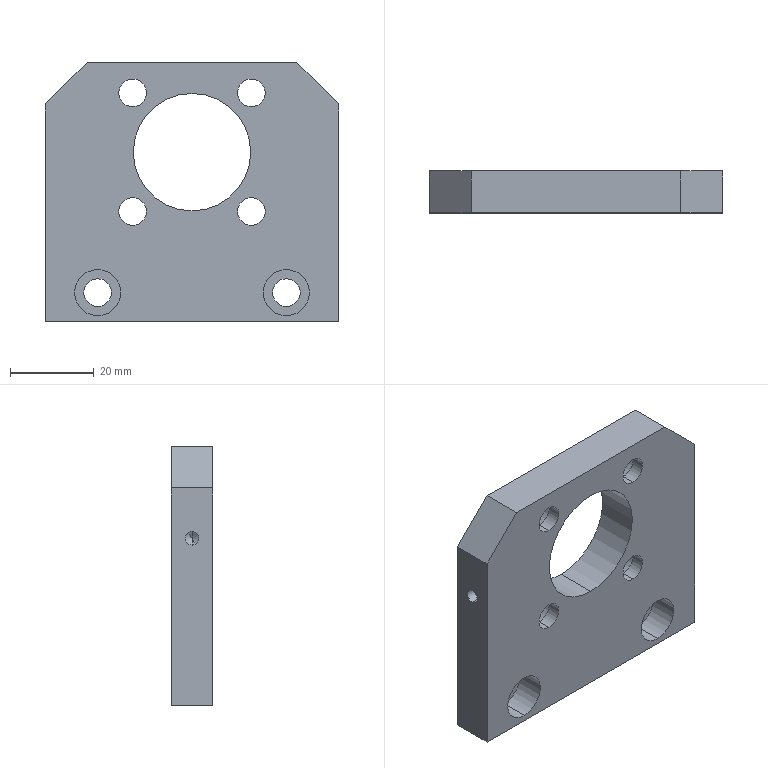Part | STEP file | PN_0045 | 1 solid | 44 faces | box 70 x 10 x 62 mm | volume 31607 mm3 | cylinder 28 | plane 14 | cone 2 | commonest cylinder face diameters 6.6 x12 11 x12 3.3 x2 28 x2